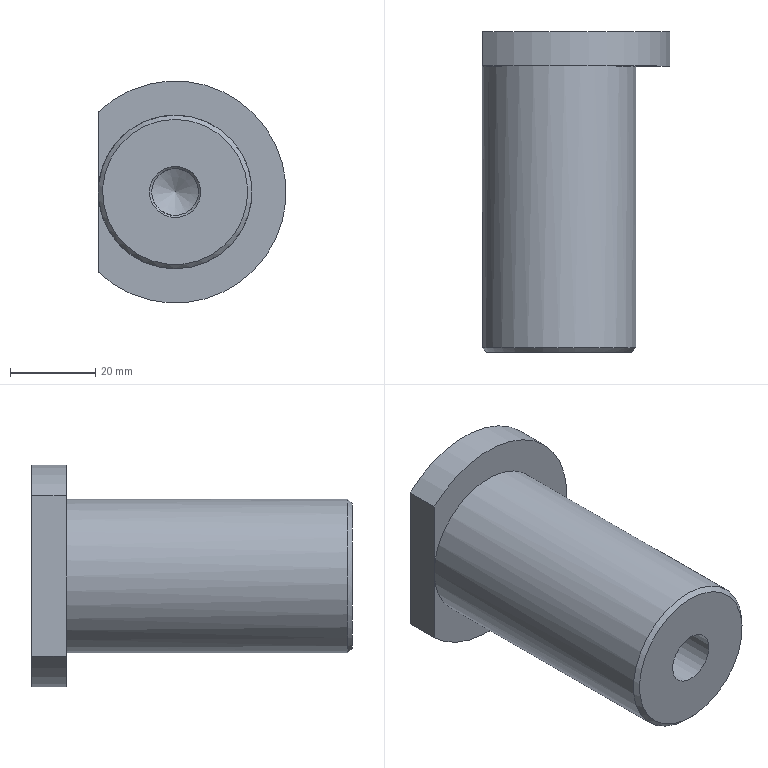Part | STEP file | EJECTION-COUPLING-SHANK_id458_x_t | 1 solid | 11 faces | box 44 x 75 x 52 mm | volume 81524 mm3 | cylinder 4 | plane 4 | cone 3 | commonest cylinder face diameters 11 x1 12 x1 36 x1 52 x1
STEP:
#1=CARTESIAN_POINT('',(0.,-275.409,0.));
#2=VERTEX_POINT('',#1);
#3=VERTEX_LOOP('',#2);
#4=FACE_BOUND('',#3,.T.);
#5=CARTESIAN_POINT('',(0.,-278.585,-5.5));
#6=VERTEX_POINT('',#5);
#7=CARTESIAN_POINT('',(0.,-278.585,0.));
#8=DIRECTION('',(0.,-1.,0.));
#9=DIRECTION('',(0.,0.,-1.));
#10=AXIS2_PLACEMENT_3D('',#7,#8,#9);
#11=CIRCLE('',#10,5.5);
#12=EDGE_CURVE('',#6,#6,#11,.T.);
#13=ORIENTED_EDGE('',*,*,#12,.T.);
#14=EDGE_LOOP('',(#13));
#15=FACE_BOUND('',#14,.T.);
#16=CARTESIAN_POINT('',(0.,-278.585,0.));
#17=DIRECTION('',(0.,-1.,0.));
#18=DIRECTION('',(0.,0.,-1.));
#19=AXIS2_PLACEMENT_3D('',#16,#17,#18);
#20=CONICAL_SURFACE('',#19,5.5,60.);
#21=ADVANCED_FACE('',(#4,#15),#20,.F.);
#22=ORIENTED_EDGE('',*,*,#12,.F.);
#23=EDGE_LOOP('',(#22));
#24=FACE_BOUND('',#23,.T.);
#25=CARTESIAN_POINT('',(-5.5,-281.864,0.));
#26=VERTEX_POINT('',#25);
#27=CARTESIAN_POINT('',(0.,-281.864,0.));
#28=DIRECTION('',(0.,-1.,0.));
#29=DIRECTION('',(-1.,0.,0.));
#30=AXIS2_PLACEMENT_3D('',#27,#28,#29);
#31=CIRCLE('',#30,5.5);
#32=EDGE_CURVE('',#26,#26,#31,.T.);
#33=ORIENTED_EDGE('',*,*,#32,.T.);
#34=EDGE_LOOP('',(#33));
#35=FACE_BOUND('',#34,.T.);
#36=CARTESIAN_POINT('',(0.,-216.75,0.));
#37=DIRECTION('',(0.,-1.,0.));
#38=DIRECTION('',(0.,0.,-1.));
#39=AXIS2_PLACEMENT_3D('',#36,#37,#38);
#40=CYLINDRICAL_SURFACE('',#39,5.5);
#41=ADVANCED_FACE('',(#24,#35),#40,.F.);
#42=ORIENTED_EDGE('',*,*,#32,.F.);
#43=EDGE_LOOP('',(#42));
#44=FACE_BOUND('',#43,.T.);
#45=CARTESIAN_POINT('',(0.,-282.364,-6.));
#46=VERTEX_POINT('',#45);
#47=CARTESIAN_POINT('',(0.,-282.364,0.));
#48=DIRECTION('',(0.,-1.,0.));
#49=DIRECTION('',(0.,0.,-1.));
#50=AXIS2_PLACEMENT_3D('',#47,#48,#49);
#51=CIRCLE('',#50,6.);
#52=EDGE_CURVE('',#46,#46,#51,.T.);
#53=ORIENTED_EDGE('',*,*,#52,.T.);
#54=EDGE_LOOP('',(#53));
#55=FACE_BOUND('',#54,.T.);
#56=CARTESIAN_POINT('',(0.,-282.364,0.));
#57=DIRECTION('',(0.,-1.,0.));
#58=DIRECTION('',(0.,0.,-1.));
#59=AXIS2_PLACEMENT_3D('',#56,#57,#58);
#60=CONICAL_SURFACE('',#59,6.,45.);
#61=ADVANCED_FACE('',(#44,#55),#60,.F.);
#62=ORIENTED_EDGE('',*,*,#52,.F.);
#63=EDGE_LOOP('',(#62));
#64=FACE_BOUND('',#63,.T.);
#65=CARTESIAN_POINT('',(0.,-295.5,-6.));
#66=VERTEX_POINT('',#65);
#67=CARTESIAN_POINT('',(0.,-295.5,0.));
#68=DIRECTION('',(0.,1.,0.));
#69=DIRECTION('',(0.,0.,-1.));
#70=AXIS2_PLACEMENT_3D('',#67,#68,#69);
#71=CIRCLE('',#70,6.);
#72=EDGE_CURVE('',#66,#66,#71,.T.);
#73=ORIENTED_EDGE('',*,*,#72,.F.);
#74=EDGE_LOOP('',(#73));
#75=FACE_BOUND('',#74,.T.);
#76=CARTESIAN_POINT('',(0.,-216.75,0.));
#77=DIRECTION('',(0.,-1.,0.));
#78=DIRECTION('',(0.,0.,-1.));
#79=AXIS2_PLACEMENT_3D('',#76,#77,#78);
#80=CYLINDRICAL_SURFACE('',#79,6.);
#81=ADVANCED_FACE('',(#64,#75),#80,.F.);
#82=CARTESIAN_POINT('',(-18.,-220.5,-18.762));
#83=VERTEX_POINT('',#82);
#84=CARTESIAN_POINT('',(-18.,-220.5,18.762));
#85=VERTEX_POINT('',#84);
#86=CARTESIAN_POINT('',(-18.,-220.5,18.762));
#87=DIRECTION('',(0.,0.,1.));
#88=VECTOR('',#87,1.);
#89=LINE('',#86,#88);
#90=EDGE_CURVE('',#83,#85,#89,.T.);
#91=ORIENTED_EDGE('',*,*,#90,.F.);
#92=CARTESIAN_POINT('',(0.,-220.5,0.));
#93=DIRECTION('',(0.,-1.,0.));
#94=DIRECTION('',(0.,0.,-1.));
#95=AXIS2_PLACEMENT_3D('',#92,#93,#94);
#96=CIRCLE('',#95,26.);
#97=EDGE_CURVE('',#83,#85,#96,.T.);
#98=ORIENTED_EDGE('',*,*,#97,.T.);
#99=EDGE_LOOP('',(#91,#98));
#100=FACE_OUTER_BOUND('',#99,.T.);
#101=CARTESIAN_POINT('',(0.,-220.5,0.));
#102=DIRECTION('',(0.,-1.,0.));
#103=DIRECTION('',(0.,0.,-1.));
#104=AXIS2_PLACEMENT_3D('',#101,#102,#103);
#105=PLANE('',#104);
#106=ADVANCED_FACE('',(#100),#105,.T.);
#107=ORIENTED_EDGE('',*,*,#72,.T.);
#108=EDGE_LOOP('',(#107));
#109=FACE_BOUND('',#108,.T.);
#110=CARTESIAN_POINT('',(0.,-295.5,17.));
#111=VERTEX_POINT('',#110);
#112=CARTESIAN_POINT('',(0.,-295.5,0.));
#113=DIRECTION('',(0.,1.,0.));
#114=DIRECTION('',(0.,0.,1.));
#115=AXIS2_PLACEMENT_3D('',#112,#113,#114);
#116=CIRCLE('',#115,17.);
#117=EDGE_CURVE('',#111,#111,#116,.T.);
#118=ORIENTED_EDGE('',*,*,#117,.F.);
#119=EDGE_LOOP('',(#118));
#120=FACE_BOUND('',#119,.T.);
#121=CARTESIAN_POINT('',(0.,-295.5,0.));
#122=DIRECTION('',(0.,-1.,0.));
#123=DIRECTION('',(0.,0.,-1.));
#124=AXIS2_PLACEMENT_3D('',#121,#122,#123);
#125=PLANE('',#124);
#126=ADVANCED_FACE('',(#109,#120),#125,.T.);
#127=CARTESIAN_POINT('',(-18.,-228.5,-18.762));
#128=VERTEX_POINT('',#127);
#129=CARTESIAN_POINT('',(-18.,-220.5,-18.762));
#130=DIRECTION('',(0.,1.,0.));
#131=VECTOR('',#130,1.);
#132=LINE('',#129,#131);
#133=EDGE_CURVE('',#128,#83,#132,.T.);
#134=ORIENTED_EDGE('',*,*,#133,.F.);
#135=CARTESIAN_POINT('',(-18.,-228.5,18.762));
#136=VERTEX_POINT('',#135);
#137=CARTESIAN_POINT('',(0.,-228.5,0.));
#138=DIRECTION('',(0.,1.,0.));
#139=DIRECTION('',(0.,0.,-1.));
#140=AXIS2_PLACEMENT_3D('',#137,#138,#139);
#141=CIRCLE('',#140,26.);
#142=EDGE_CURVE('',#136,#128,#141,.T.);
#143=ORIENTED_EDGE('',*,*,#142,.F.);
#144=CARTESIAN_POINT('',(-18.,-220.5,18.762));
#145=DIRECTION('',(0.,-1.,0.));
#146=VECTOR('',#145,1.);
#147=LINE('',#144,#146);
#148=EDGE_CURVE('',#85,#136,#147,.T.);
#149=ORIENTED_EDGE('',*,*,#148,.F.);
#150=ORIENTED_EDGE('',*,*,#97,.F.);
#151=EDGE_LOOP('',(#134,#143,#149,#150));
#152=FACE_OUTER_BOUND('',#151,.T.);
#153=CARTESIAN_POINT('',(0.,-216.75,0.));
#154=DIRECTION('',(0.,-1.,0.));
#155=DIRECTION('',(0.,0.,-1.));
#156=AXIS2_PLACEMENT_3D('',#153,#154,#155);
#157=CYLINDRICAL_SURFACE('',#156,26.);
#158=ADVANCED_FACE('',(#152),#157,.F.);
#159=ORIENTED_EDGE('',*,*,#90,.T.);
#160=ORIENTED_EDGE('',*,*,#148,.T.);
#161=CARTESIAN_POINT('',(-18.,-228.5,0.));
#162=DIRECTION('',(0.,0.,1.));
#163=VECTOR('',#162,1.);
#164=LINE('',#161,#163);
#165=EDGE_CURVE('',#128,#136,#164,.T.);
#166=ORIENTED_EDGE('',*,*,#165,.F.);
#167=ORIENTED_EDGE('',*,*,#133,.T.);
#168=EDGE_LOOP('',(#159,#160,#166,#167));
#169=FACE_OUTER_BOUND('',#168,.T.);
#170=CARTESIAN_POINT('',(-18.,-220.5,18.762));
#171=DIRECTION('',(1.,0.,0.));
#172=DIRECTION('',(0.,0.,-1.));
#173=AXIS2_PLACEMENT_3D('',#170,#171,#172);
#174=PLANE('',#173);
#175=ADVANCED_FACE('',(#169),#174,.T.);
#176=ORIENTED_EDGE('',*,*,#117,.T.);
#177=EDGE_LOOP('',(#176));
#178=FACE_BOUND('',#177,.T.);
#179=CARTESIAN_POINT('',(0.,-294.5,-18.));
#180=VERTEX_POINT('',#179);
#181=CARTESIAN_POINT('',(0.,-294.5,0.));
#182=DIRECTION('',(0.,1.,0.));
#183=DIRECTION('',(0.,0.,-1.));
#184=AXIS2_PLACEMENT_3D('',#181,#182,#183);
#185=CIRCLE('',#184,18.);
#186=EDGE_CURVE('',#180,#180,#185,.T.);
#187=ORIENTED_EDGE('',*,*,#186,.F.);
#188=EDGE_LOOP('',(#187));
#189=FACE_BOUND('',#188,.T.);
#190=CARTESIAN_POINT('',(0.,-294.5,0.));
#191=DIRECTION('',(0.,1.,0.));
#192=DIRECTION('',(0.,0.,1.));
#193=AXIS2_PLACEMENT_3D('',#190,#191,#192);
#194=CONICAL_SURFACE('',#193,18.,45.);
#195=ADVANCED_FACE('',(#178,#189),#194,.T.);
#196=ORIENTED_EDGE('',*,*,#142,.T.);
#197=ORIENTED_EDGE('',*,*,#165,.T.);
#198=EDGE_LOOP('',(#196,#197));
#199=FACE_BOUND('',#198,.T.);
#200=CARTESIAN_POINT('',(0.,-228.5,-18.));
#201=VERTEX_POINT('',#200);
#202=CARTESIAN_POINT('',(0.,-228.5,0.));
#203=DIRECTION('',(0.,-1.,0.));
#204=DIRECTION('',(0.,0.,-1.));
#205=AXIS2_PLACEMENT_3D('',#202,#203,#204);
#206=CIRCLE('',#205,18.);
#207=EDGE_CURVE('',#201,#201,#206,.T.);
#208=ORIENTED_EDGE('',*,*,#207,.F.);
#209=EDGE_LOOP('',(#208));
#210=FACE_BOUND('',#209,.T.);
#211=CARTESIAN_POINT('',(0.,-228.5,0.));
#212=DIRECTION('',(0.,-1.,0.));
#213=DIRECTION('',(0.,0.,-1.));
#214=AXIS2_PLACEMENT_3D('',#211,#212,#213);
#215=PLANE('',#214);
#216=ADVANCED_FACE('',(#199,#210),#215,.T.);
#217=ORIENTED_EDGE('',*,*,#186,.T.);
#218=EDGE_LOOP('',(#217));
#219=FACE_BOUND('',#218,.T.);
#220=ORIENTED_EDGE('',*,*,#207,.T.);
#221=EDGE_LOOP('',(#220));
#222=FACE_BOUND('',#221,.T.);
#223=CARTESIAN_POINT('',(0.,-216.75,0.));
#224=DIRECTION('',(0.,-1.,0.));
#225=DIRECTION('',(0.,0.,-1.));
#226=AXIS2_PLACEMENT_3D('',#223,#224,#225);
#227=CYLINDRICAL_SURFACE('',#226,18.);
#228=ADVANCED_FACE('',(#219,#222),#227,.T.);
#229=CLOSED_SHELL('',(#21,#41,#61,#81,#106,#126,#158,#175,#195,#216,#228));
#230=MANIFOLD_SOLID_BREP('',#229);
#231=(LENGTH_UNIT()NAMED_UNIT(*)SI_UNIT(.MILLI.,.METRE.));
#232=UNCERTAINTY_MEASURE_WITH_UNIT(LENGTH_MEASURE(0.00004123),#231,'','');
#233=(NAMED_UNIT(*)PLANE_ANGLE_UNIT()SI_UNIT($,.RADIAN.));
#234=PLANE_ANGLE_MEASURE_WITH_UNIT(PLANE_ANGLE_MEASURE(0.01745),#233);
#235=DIMENSIONAL_EXPONENTS(0.,0.,0.,0.,0.,0.,0.);
#236=(CONVERSION_BASED_UNIT('DEGREE',#234)NAMED_UNIT(#235)PLANE_ANGLE_UNIT());
#237=(NAMED_UNIT(*)SI_UNIT($,.STERADIAN.)SOLID_ANGLE_UNIT());
#238=(GEOMETRIC_REPRESENTATION_CONTEXT(3)GLOBAL_UNCERTAINTY_ASSIGNED_CONTEXT((#232))GLOBAL_UNIT_ASSIGNED_CONTEXT((#231,#236,#237))REPRESENTATION_CONTEXT('',''));
#239=ADVANCED_BREP_SHAPE_REPRESENTATION('',(#230),#238);